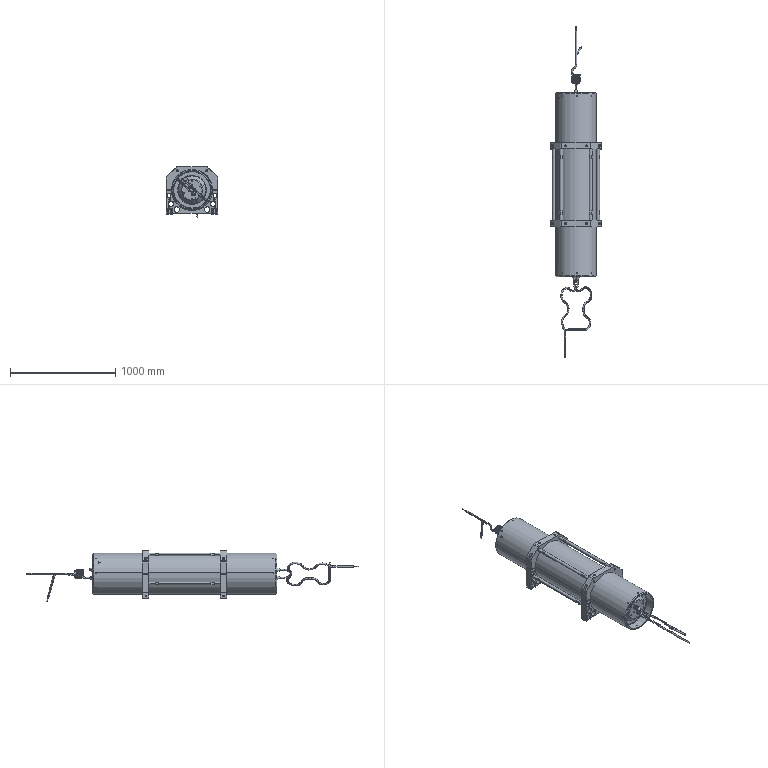Part | NX | features BREP 18 | 31 solids | 2453 faces | box 490 x 3159 x 484.108 mm | volume 97459256 mm3 | cylinder 795 | cone 543 | plane 501 | spline 398 | torus 210 | sphere 6 | commonest cylinder face diameters 30 x144 26 x104 6.35 x37 6.8 x36 4.2 x32 10.2 x32